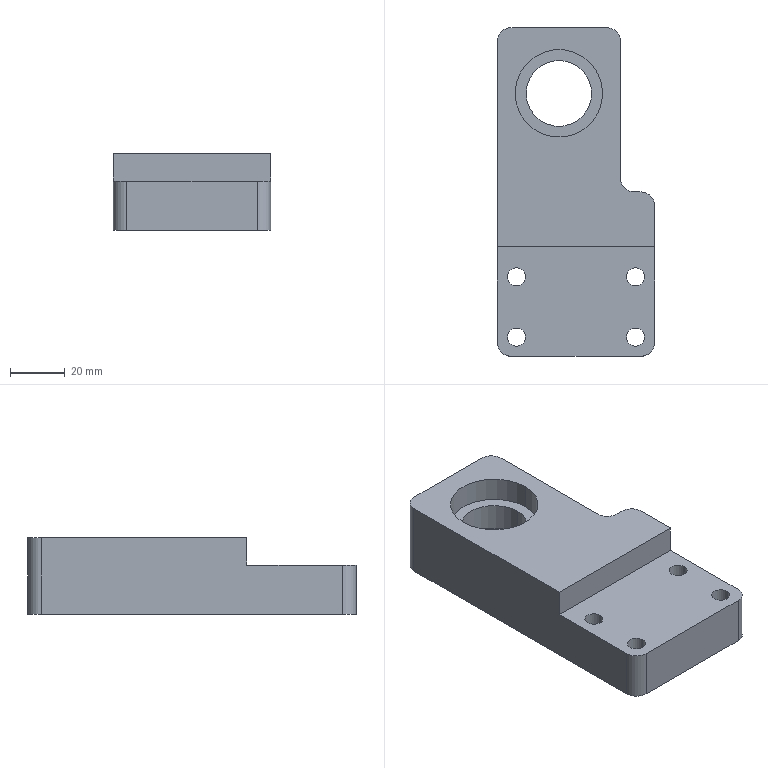Part | STEP file | 10000020597swp000-1 | 1 solid | 58 faces | box 57.5 x 120 x 28 mm | volume 124322 mm3 | cylinder 36 | plane 18 | cone 4 | commonest cylinder face diameters 6.6 x8 11 x8 10 x6 2.5 x4 5 x4 32 x4